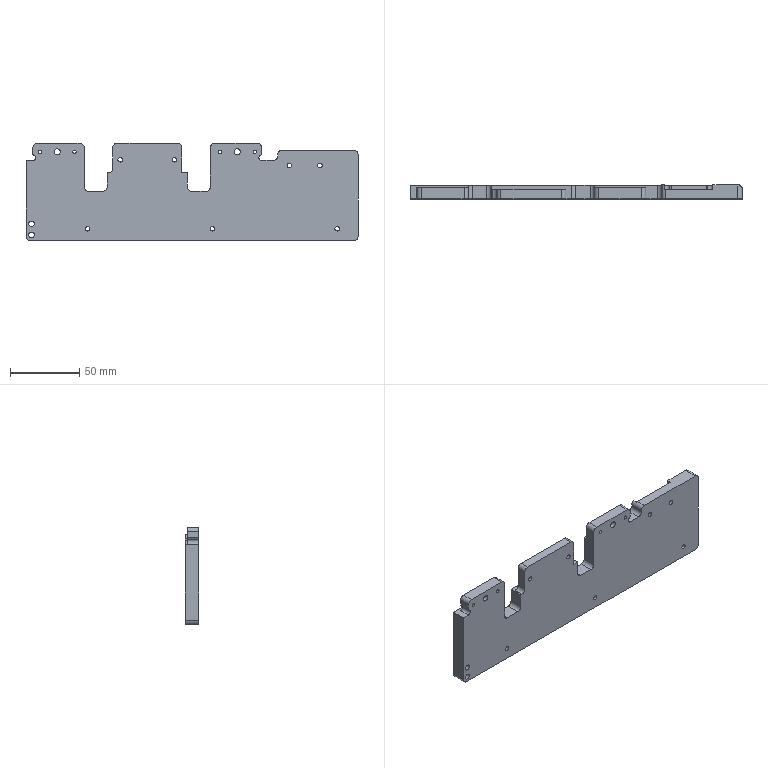Part | 1 solid | 80 faces | box 239.5 x 10 x 70 mm | volume 139716 mm3 | cylinder 44 | plane 33 | cone 3 | commonest cylinder face diameters 6 x16 3.3 x10 4 x6 2 x4 2.5 x4 4.5 x2